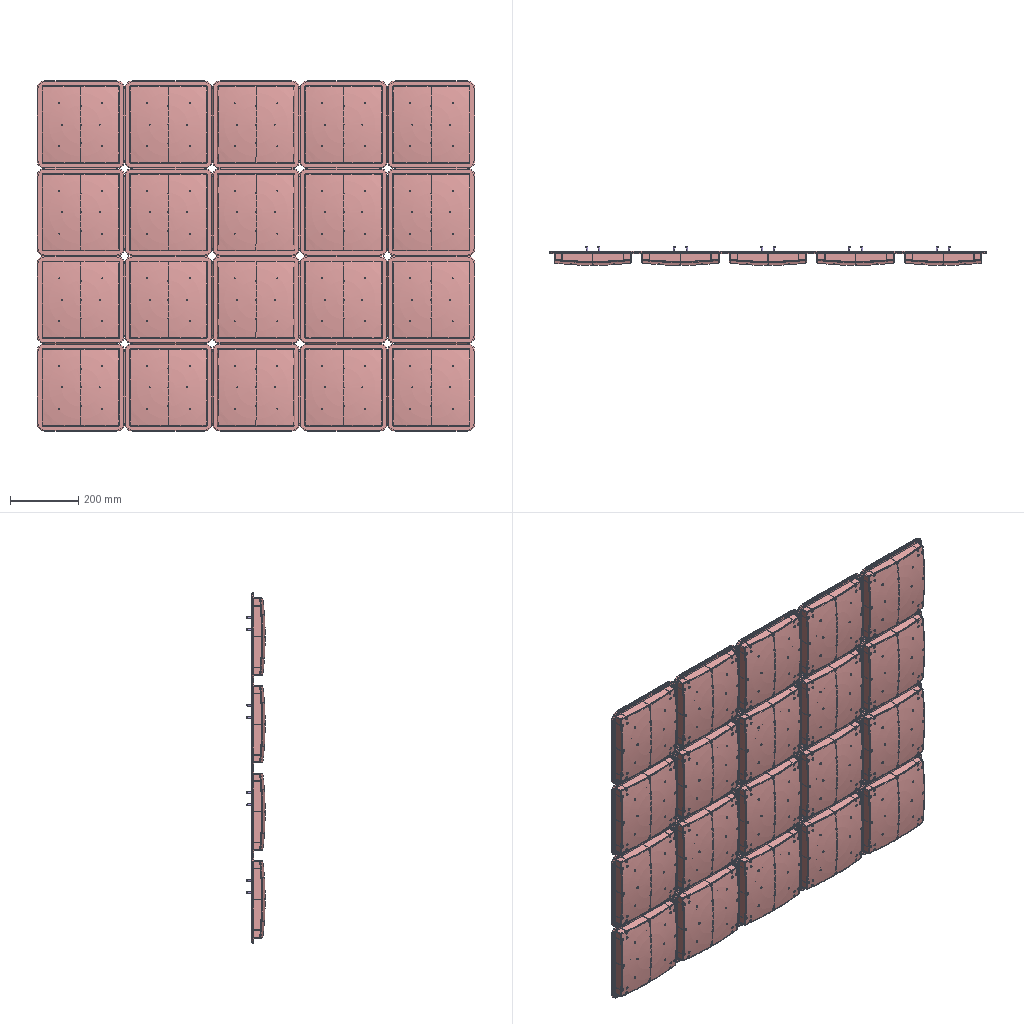Assembly | SolidWorks | 7 different items | 121 placed | box 1285 x 54 x 1028 mm
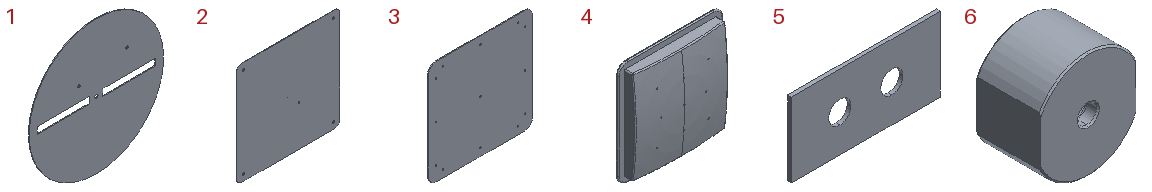Parts list (item | name | quantity | size | volume | features):
1 | - | x20 | 165 x 1 x 165 mm | 20280 mm3 | features Extrusion 1
2 | - | x20 | 206 x 18.5 x 206 mm | 42483 mm3 | features Chamfer 2, Extrusion 1, Helix 1, ICE 1, SweepCut 1
3 | - | x20 | 249.5 x 17 x 249.5 mm | 125056 mm3 | features Chamfer 2, Extrusion 1, ICE 1
4 | - | x20 | 257 x 39.299 x 257 mm | 199680 mm3 | features ICE 6, Fillet 2, RevCut 2, 3DProfileFeature 1, Extrusion 1, Rib 1, Shell 1, SketchPattern 1
5 | - | x20 | 20 x 0.5 x 10 mm | 92.931 mm3 | features Extrusion 1
6 | - | x20 | 12.5 x 8.5 x 14.1 mm | 1218 mm3 | features Chamfer 1, Extrusion 1, Helix 1, SweepCut 1
7 | oval head semi-tubular rivets gb | x1 | - | - | -
Mates (type | each side: item.copy, entity, surface, feature):
Coordinate | 4.1 select_type:25 | assembly select_type:11
Coincident | 2.1 plane | assembly plane | 2 times
Coincident | 4.1 face plane Boss-Extrude5 | 2.1 face plane Boss-Extrude1
Concentric | 2.1 edge | 1.1 edge
DistanceDim | 1.1 face plane Boss-Extrude1 | 2.1 face plane Boss-Extrude1
Concentric | 2.1 face cylinder Boss-Extrude1 | 1.1 face cylinder Boss-Extrude1
Concentric | 1.1 edge | 6.1 edge
Coincident | 1.1 face plane Boss-Extrude1 | 6.1 face plane Boss-Extrude1
Coincident | 2.1 face plane Boss-Extrude1 | 5.1 face plane Boss-Extrude1
Coincident | 3.1 plane | assembly plane | 2 times
Coincident | 4.1 face plane Boss-Extrude3 | 3.1 face plane Boss-Extrude1